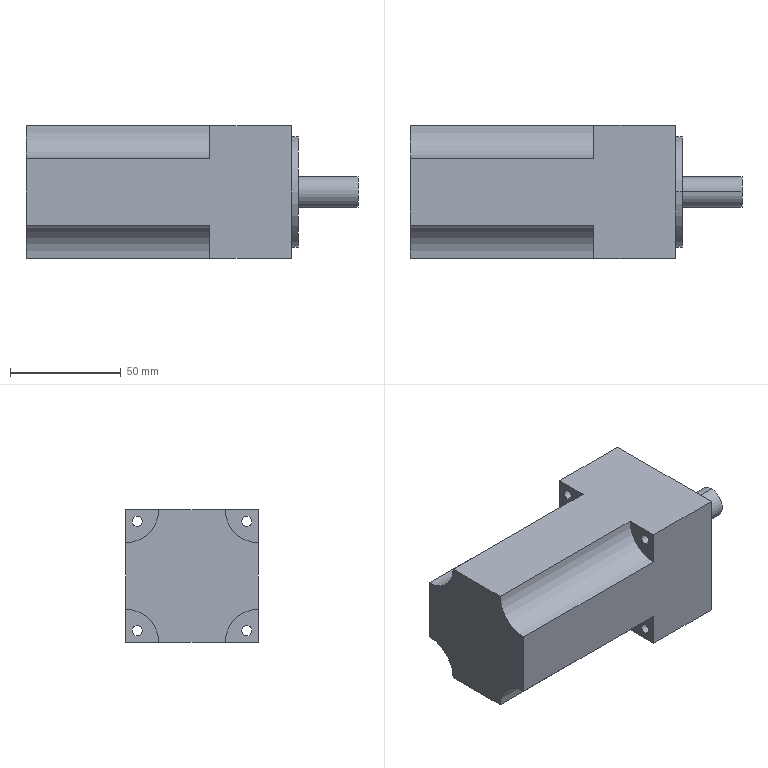Part | STEP file | PN_0048 MSMD042G | 1 solid | 28 faces | box 150 x 60 x 60 mm | volume 380918 mm3 | cylinder 16 | plane 12 | commonest cylinder face diameters 4.6 x8 30 x4 14 x2 50 x2